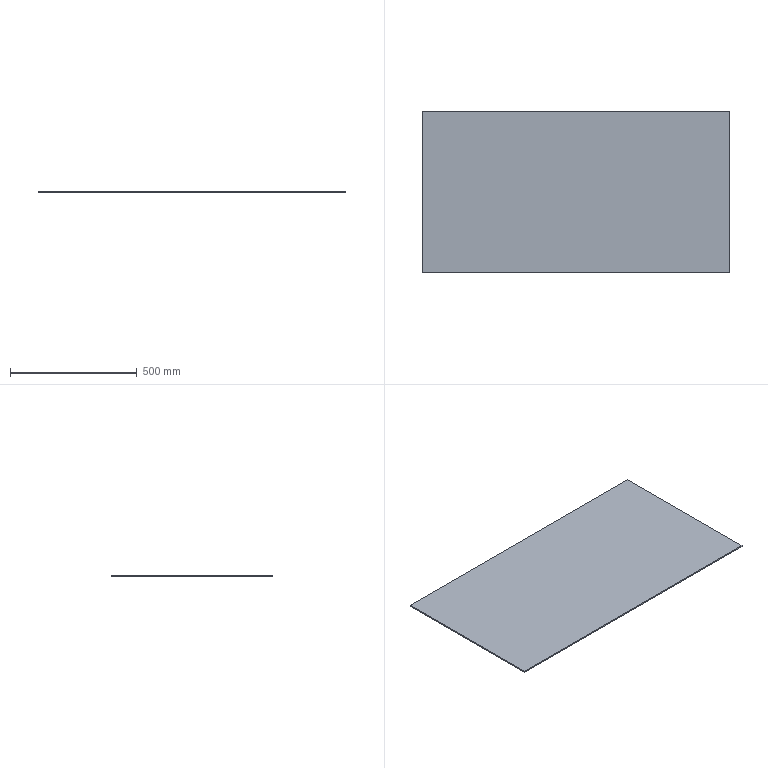Part | SolidWorks | features Extrusion 1 | 1 solid | 6 faces | box 1216 x 639 x 5 mm | volume 3885120 mm3 | plane 6
STEP:
#1=CARTESIAN_POINT('',(608.,-319.5,0.));
#2=VERTEX_POINT('',#1);
#3=CARTESIAN_POINT('',(608.,319.5,0.));
#4=VERTEX_POINT('',#3);
#5=CARTESIAN_POINT('',(608.,319.5,0.));
#6=DIRECTION('',(0.,1.,0.));
#7=VECTOR('',#6,1000.);
#8=LINE('',#5,#7);
#9=EDGE_CURVE('',#2,#4,#8,.T.);
#10=ORIENTED_EDGE('',*,*,#9,.T.);
#11=CARTESIAN_POINT('',(608.,319.5,5.));
#12=VERTEX_POINT('',#11);
#13=CARTESIAN_POINT('',(608.,319.5,5.));
#14=DIRECTION('',(0.,0.,-1.));
#15=VECTOR('',#14,1000.);
#16=LINE('',#13,#15);
#17=EDGE_CURVE('',#12,#4,#16,.T.);
#18=ORIENTED_EDGE('',*,*,#17,.F.);
#19=CARTESIAN_POINT('',(608.,-319.5,5.));
#20=VERTEX_POINT('',#19);
#21=CARTESIAN_POINT('',(608.,319.5,5.));
#22=DIRECTION('',(0.,1.,0.));
#23=VECTOR('',#22,1000.);
#24=LINE('',#21,#23);
#25=EDGE_CURVE('',#20,#12,#24,.T.);
#26=ORIENTED_EDGE('',*,*,#25,.F.);
#27=CARTESIAN_POINT('',(608.,-319.5,5.));
#28=DIRECTION('',(0.,0.,-1.));
#29=VECTOR('',#28,1000.);
#30=LINE('',#27,#29);
#31=EDGE_CURVE('',#20,#2,#30,.T.);
#32=ORIENTED_EDGE('',*,*,#31,.T.);
#33=EDGE_LOOP('',(#10,#18,#26,#32));
#34=FACE_OUTER_BOUND('',#33,.T.);
#35=CARTESIAN_POINT('',(608.,319.5,5.));
#36=DIRECTION('',(-1.,0.,0.));
#37=DIRECTION('',(0.,0.,1.));
#38=AXIS2_PLACEMENT_3D('',#35,#36,#37);
#39=PLANE('',#38);
#40=ADVANCED_FACE('',(#34),#39,.F.);
#41=CARTESIAN_POINT('',(-608.,319.5,0.));
#42=VERTEX_POINT('',#41);
#43=CARTESIAN_POINT('',(-608.,319.5,0.));
#44=DIRECTION('',(-1.,0.,0.));
#45=VECTOR('',#44,1000.);
#46=LINE('',#43,#45);
#47=EDGE_CURVE('',#4,#42,#46,.T.);
#48=ORIENTED_EDGE('',*,*,#47,.T.);
#49=CARTESIAN_POINT('',(-608.,319.5,5.));
#50=VERTEX_POINT('',#49);
#51=CARTESIAN_POINT('',(-608.,319.5,5.));
#52=DIRECTION('',(0.,0.,-1.));
#53=VECTOR('',#52,1000.);
#54=LINE('',#51,#53);
#55=EDGE_CURVE('',#50,#42,#54,.T.);
#56=ORIENTED_EDGE('',*,*,#55,.F.);
#57=CARTESIAN_POINT('',(-608.,319.5,5.));
#58=DIRECTION('',(-1.,0.,0.));
#59=VECTOR('',#58,1000.);
#60=LINE('',#57,#59);
#61=EDGE_CURVE('',#12,#50,#60,.T.);
#62=ORIENTED_EDGE('',*,*,#61,.F.);
#63=ORIENTED_EDGE('',*,*,#17,.T.);
#64=EDGE_LOOP('',(#48,#56,#62,#63));
#65=FACE_OUTER_BOUND('',#64,.T.);
#66=CARTESIAN_POINT('',(-608.,319.5,5.));
#67=DIRECTION('',(0.,-1.,0.));
#68=DIRECTION('',(0.,0.,-1.));
#69=AXIS2_PLACEMENT_3D('',#66,#67,#68);
#70=PLANE('',#69);
#71=ADVANCED_FACE('',(#65),#70,.F.);
#72=CARTESIAN_POINT('',(-608.,-319.5,0.));
#73=VERTEX_POINT('',#72);
#74=CARTESIAN_POINT('',(-608.,319.5,0.));
#75=DIRECTION('',(0.,-1.,0.));
#76=VECTOR('',#75,1000.);
#77=LINE('',#74,#76);
#78=EDGE_CURVE('',#42,#73,#77,.T.);
#79=ORIENTED_EDGE('',*,*,#78,.T.);
#80=CARTESIAN_POINT('',(-608.,-319.5,5.));
#81=VERTEX_POINT('',#80);
#82=CARTESIAN_POINT('',(-608.,-319.5,5.));
#83=DIRECTION('',(0.,0.,-1.));
#84=VECTOR('',#83,1000.);
#85=LINE('',#82,#84);
#86=EDGE_CURVE('',#81,#73,#85,.T.);
#87=ORIENTED_EDGE('',*,*,#86,.F.);
#88=CARTESIAN_POINT('',(-608.,319.5,5.));
#89=DIRECTION('',(0.,-1.,0.));
#90=VECTOR('',#89,1000.);
#91=LINE('',#88,#90);
#92=EDGE_CURVE('',#50,#81,#91,.T.);
#93=ORIENTED_EDGE('',*,*,#92,.F.);
#94=ORIENTED_EDGE('',*,*,#55,.T.);
#95=EDGE_LOOP('',(#79,#87,#93,#94));
#96=FACE_OUTER_BOUND('',#95,.T.);
#97=CARTESIAN_POINT('',(-608.,319.5,5.));
#98=DIRECTION('',(1.,0.,0.));
#99=DIRECTION('',(0.,0.,-1.));
#100=AXIS2_PLACEMENT_3D('',#97,#98,#99);
#101=PLANE('',#100);
#102=ADVANCED_FACE('',(#96),#101,.F.);
#103=CARTESIAN_POINT('',(-608.,-319.5,0.));
#104=DIRECTION('',(1.,0.,0.));
#105=VECTOR('',#104,1000.);
#106=LINE('',#103,#105);
#107=EDGE_CURVE('',#73,#2,#106,.T.);
#108=ORIENTED_EDGE('',*,*,#107,.T.);
#109=ORIENTED_EDGE('',*,*,#31,.F.);
#110=CARTESIAN_POINT('',(-608.,-319.5,5.));
#111=DIRECTION('',(1.,0.,0.));
#112=VECTOR('',#111,1000.);
#113=LINE('',#110,#112);
#114=EDGE_CURVE('',#81,#20,#113,.T.);
#115=ORIENTED_EDGE('',*,*,#114,.F.);
#116=ORIENTED_EDGE('',*,*,#86,.T.);
#117=EDGE_LOOP('',(#108,#109,#115,#116));
#118=FACE_OUTER_BOUND('',#117,.T.);
#119=CARTESIAN_POINT('',(-608.,-319.5,5.));
#120=DIRECTION('',(0.,1.,0.));
#121=DIRECTION('',(0.,0.,1.));
#122=AXIS2_PLACEMENT_3D('',#119,#120,#121);
#123=PLANE('',#122);
#124=ADVANCED_FACE('',(#118),#123,.F.);
#125=ORIENTED_EDGE('',*,*,#25,.T.);
#126=ORIENTED_EDGE('',*,*,#61,.T.);
#127=ORIENTED_EDGE('',*,*,#92,.T.);
#128=ORIENTED_EDGE('',*,*,#114,.T.);
#129=EDGE_LOOP('',(#125,#126,#127,#128));
#130=FACE_OUTER_BOUND('',#129,.T.);
#131=CARTESIAN_POINT('',(0.,0.,5.));
#132=DIRECTION('',(0.,0.,1.));
#133=DIRECTION('',(1.,0.,0.));
#134=AXIS2_PLACEMENT_3D('',#131,#132,#133);
#135=PLANE('',#134);
#136=ADVANCED_FACE('',(#130),#135,.T.);
#137=ORIENTED_EDGE('',*,*,#9,.F.);
#138=ORIENTED_EDGE('',*,*,#107,.F.);
#139=ORIENTED_EDGE('',*,*,#78,.F.);
#140=ORIENTED_EDGE('',*,*,#47,.F.);
#141=EDGE_LOOP('',(#137,#138,#139,#140));
#142=FACE_OUTER_BOUND('',#141,.T.);
#143=CARTESIAN_POINT('',(0.,0.,0.));
#144=DIRECTION('',(0.,0.,1.));
#145=DIRECTION('',(1.,0.,0.));
#146=AXIS2_PLACEMENT_3D('',#143,#144,#145);
#147=PLANE('',#146);
#148=ADVANCED_FACE('',(#142),#147,.F.);
#149=CLOSED_SHELL('',(#40,#71,#102,#124,#136,#148));
#150=MANIFOLD_SOLID_BREP('',#149);
#151=CARTESIAN_POINT('',(0.,0.,0.));
#152=DIRECTION('',(0.,0.,1.));
#153=DIRECTION('',(1.,0.,0.));
#154=AXIS2_PLACEMENT_3D('',#151,#152,#153);
#155=(LENGTH_UNIT()NAMED_UNIT(*)SI_UNIT(.MILLI.,.METRE.));
#156=UNCERTAINTY_MEASURE_WITH_UNIT(LENGTH_MEASURE(0.00001),#155,'','');
#157=(NAMED_UNIT(*)PLANE_ANGLE_UNIT()SI_UNIT($,.RADIAN.));
#158=(NAMED_UNIT(*)SI_UNIT($,.STERADIAN.)SOLID_ANGLE_UNIT());
#159=(GEOMETRIC_REPRESENTATION_CONTEXT(3)GLOBAL_UNCERTAINTY_ASSIGNED_CONTEXT((#156))GLOBAL_UNIT_ASSIGNED_CONTEXT((#155,#157,#158))REPRESENTATION_CONTEXT('',''));
#160=ADVANCED_BREP_SHAPE_REPRESENTATION('',(#150,#154),#159);